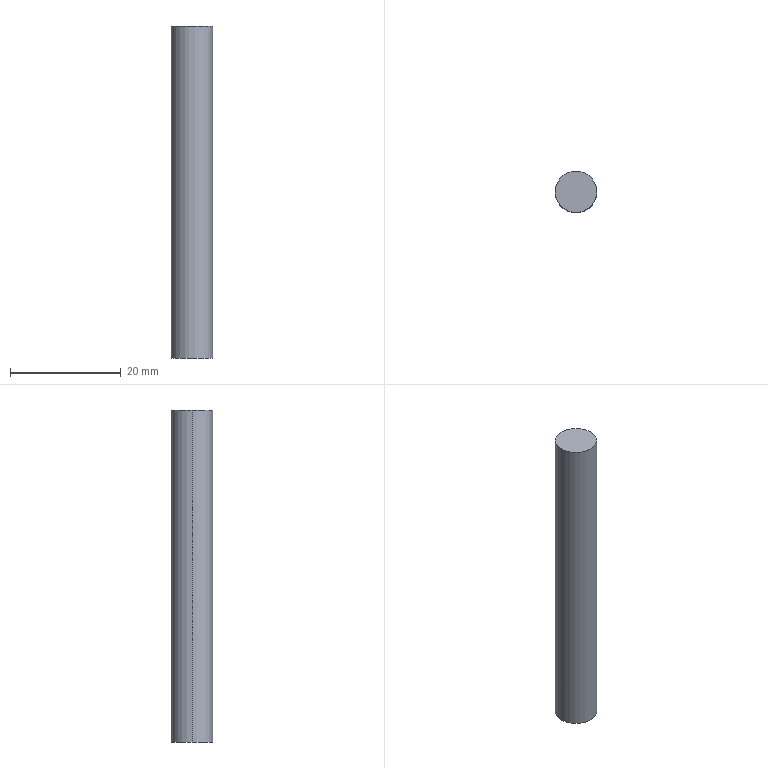Part | SolidWorks | features BaseBody 1 | 1 solid | 4 faces | box 7.5 x 7.5 x 60 mm | volume 2651 mm3 | cylinder 2 | plane 2 | commonest cylinder face diameters 7.5 x2
STEP:
#1=CARTESIAN_POINT('',(-3.75,0.,0.));
#2=VERTEX_POINT('',#1);
#3=CARTESIAN_POINT('',(3.75,0.,0.));
#4=VERTEX_POINT('',#3);
#5=CARTESIAN_POINT('',(0.,0.,0.));
#6=DIRECTION('',(0.,0.,-1.));
#7=DIRECTION('',(-1.,0.,0.));
#8=AXIS2_PLACEMENT_3D('',#5,#6,#7);
#9=CIRCLE('',#8,3.75);
#10=EDGE_CURVE('',#2,#4,#9,.T.);
#11=ORIENTED_EDGE('',*,*,#10,.T.);
#12=CARTESIAN_POINT('',(3.75,0.,-60.));
#13=VERTEX_POINT('',#12);
#14=CARTESIAN_POINT('',(3.75,0.,-60.));
#15=DIRECTION('',(0.,0.,-1.));
#16=VECTOR('',#15,1000.);
#17=LINE('',#14,#16);
#18=EDGE_CURVE('',#4,#13,#17,.T.);
#19=ORIENTED_EDGE('',*,*,#18,.T.);
#20=CARTESIAN_POINT('',(-3.75,0.,-60.));
#21=VERTEX_POINT('',#20);
#22=CARTESIAN_POINT('',(0.,0.,-60.));
#23=DIRECTION('',(0.,0.,1.));
#24=DIRECTION('',(-1.,0.,0.));
#25=AXIS2_PLACEMENT_3D('',#22,#23,#24);
#26=CIRCLE('',#25,3.75);
#27=EDGE_CURVE('',#13,#21,#26,.T.);
#28=ORIENTED_EDGE('',*,*,#27,.T.);
#29=CARTESIAN_POINT('',(-3.75,0.,-60.));
#30=DIRECTION('',(0.,0.,-1.));
#31=VECTOR('',#30,1000.);
#32=LINE('',#29,#31);
#33=EDGE_CURVE('',#2,#21,#32,.T.);
#34=ORIENTED_EDGE('',*,*,#33,.F.);
#35=EDGE_LOOP('',(#11,#19,#28,#34));
#36=FACE_OUTER_BOUND('',#35,.T.);
#37=CARTESIAN_POINT('',(0.,0.,-60.));
#38=DIRECTION('',(0.,0.,-1.));
#39=DIRECTION('',(-1.,0.,0.));
#40=AXIS2_PLACEMENT_3D('',#37,#38,#39);
#41=CYLINDRICAL_SURFACE('',#40,3.75);
#42=ADVANCED_FACE('',(#36),#41,.T.);
#43=ORIENTED_EDGE('',*,*,#18,.F.);
#44=CARTESIAN_POINT('',(0.,0.,0.));
#45=DIRECTION('',(0.,0.,-1.));
#46=DIRECTION('',(-1.,0.,0.));
#47=AXIS2_PLACEMENT_3D('',#44,#45,#46);
#48=CIRCLE('',#47,3.75);
#49=EDGE_CURVE('',#4,#2,#48,.T.);
#50=ORIENTED_EDGE('',*,*,#49,.T.);
#51=ORIENTED_EDGE('',*,*,#33,.T.);
#52=CARTESIAN_POINT('',(0.,0.,-60.));
#53=DIRECTION('',(0.,0.,1.));
#54=DIRECTION('',(-1.,0.,0.));
#55=AXIS2_PLACEMENT_3D('',#52,#53,#54);
#56=CIRCLE('',#55,3.75);
#57=EDGE_CURVE('',#21,#13,#56,.T.);
#58=ORIENTED_EDGE('',*,*,#57,.T.);
#59=EDGE_LOOP('',(#43,#50,#51,#58));
#60=FACE_OUTER_BOUND('',#59,.T.);
#61=CARTESIAN_POINT('',(0.,0.,-60.));
#62=DIRECTION('',(0.,0.,-1.));
#63=DIRECTION('',(-1.,0.,0.));
#64=AXIS2_PLACEMENT_3D('',#61,#62,#63);
#65=CYLINDRICAL_SURFACE('',#64,3.75);
#66=ADVANCED_FACE('',(#60),#65,.T.);
#67=ORIENTED_EDGE('',*,*,#57,.F.);
#68=ORIENTED_EDGE('',*,*,#27,.F.);
#69=EDGE_LOOP('',(#67,#68));
#70=FACE_OUTER_BOUND('',#69,.T.);
#71=CARTESIAN_POINT('',(0.,0.,-60.));
#72=DIRECTION('',(0.,0.,-1.));
#73=DIRECTION('',(-1.,0.,0.));
#74=AXIS2_PLACEMENT_3D('',#71,#72,#73);
#75=PLANE('',#74);
#76=ADVANCED_FACE('',(#70),#75,.T.);
#77=ORIENTED_EDGE('',*,*,#10,.F.);
#78=ORIENTED_EDGE('',*,*,#49,.F.);
#79=EDGE_LOOP('',(#77,#78));
#80=FACE_OUTER_BOUND('',#79,.T.);
#81=CARTESIAN_POINT('',(0.,0.,0.));
#82=DIRECTION('',(0.,0.,-1.));
#83=DIRECTION('',(-1.,0.,0.));
#84=AXIS2_PLACEMENT_3D('',#81,#82,#83);
#85=PLANE('',#84);
#86=ADVANCED_FACE('',(#80),#85,.F.);
#87=CLOSED_SHELL('',(#42,#66,#76,#86));
#88=MANIFOLD_SOLID_BREP('',#87);
#89=CARTESIAN_POINT('',(0.,0.,0.));
#90=DIRECTION('',(0.,0.,1.));
#91=DIRECTION('',(1.,0.,0.));
#92=AXIS2_PLACEMENT_3D('',#89,#90,#91);
#93=(LENGTH_UNIT()NAMED_UNIT(*)SI_UNIT(.MILLI.,.METRE.));
#94=UNCERTAINTY_MEASURE_WITH_UNIT(LENGTH_MEASURE(0.00001),#93,'','');
#95=(NAMED_UNIT(*)PLANE_ANGLE_UNIT()SI_UNIT($,.RADIAN.));
#96=(NAMED_UNIT(*)SI_UNIT($,.STERADIAN.)SOLID_ANGLE_UNIT());
#97=(GEOMETRIC_REPRESENTATION_CONTEXT(3)GLOBAL_UNCERTAINTY_ASSIGNED_CONTEXT((#94))GLOBAL_UNIT_ASSIGNED_CONTEXT((#93,#95,#96))REPRESENTATION_CONTEXT('',''));
#98=ADVANCED_BREP_SHAPE_REPRESENTATION('',(#88,#92),#97);